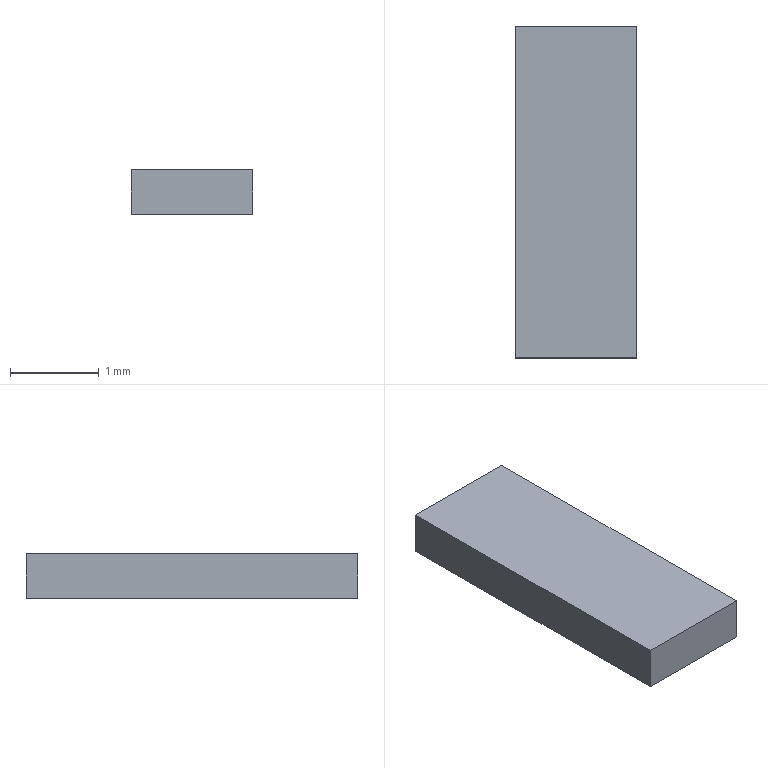Part | SolidWorks | features BaseBody 1 | 1 solid | 6 faces | box 1.375 x 3.75 x 0.5 mm | volume 2.578 mm3 | plane 6
STEP:
#1=CARTESIAN_POINT('',(-6.625,18.625,1.));
#2=VERTEX_POINT('',#1);
#3=CARTESIAN_POINT('',(-6.625,14.875,1.));
#4=VERTEX_POINT('',#3);
#5=CARTESIAN_POINT('',(-6.625,18.625,1.));
#6=DIRECTION('',(0.,-1.,0.));
#7=VECTOR('',#6,1000.);
#8=LINE('',#5,#7);
#9=EDGE_CURVE('',#2,#4,#8,.T.);
#10=ORIENTED_EDGE('',*,*,#9,.T.);
#11=CARTESIAN_POINT('',(-6.625,14.875,1.5));
#12=VERTEX_POINT('',#11);
#13=CARTESIAN_POINT('',(-6.625,14.875,1.5));
#14=DIRECTION('',(0.,0.,-1.));
#15=VECTOR('',#14,1000.);
#16=LINE('',#13,#15);
#17=EDGE_CURVE('',#12,#4,#16,.T.);
#18=ORIENTED_EDGE('',*,*,#17,.F.);
#19=CARTESIAN_POINT('',(-6.625,18.625,1.5));
#20=VERTEX_POINT('',#19);
#21=CARTESIAN_POINT('',(-6.625,18.625,1.5));
#22=DIRECTION('',(0.,-1.,0.));
#23=VECTOR('',#22,1000.);
#24=LINE('',#21,#23);
#25=EDGE_CURVE('',#20,#12,#24,.T.);
#26=ORIENTED_EDGE('',*,*,#25,.F.);
#27=CARTESIAN_POINT('',(-6.625,18.625,1.5));
#28=DIRECTION('',(0.,0.,-1.));
#29=VECTOR('',#28,1000.);
#30=LINE('',#27,#29);
#31=EDGE_CURVE('',#20,#2,#30,.T.);
#32=ORIENTED_EDGE('',*,*,#31,.T.);
#33=EDGE_LOOP('',(#10,#18,#26,#32));
#34=FACE_OUTER_BOUND('',#33,.T.);
#35=CARTESIAN_POINT('',(-6.625,18.625,1.5));
#36=DIRECTION('',(1.,0.,0.));
#37=DIRECTION('',(0.,0.,-1.));
#38=AXIS2_PLACEMENT_3D('',#35,#36,#37);
#39=PLANE('',#38);
#40=ADVANCED_FACE('',(#34),#39,.F.);
#41=CARTESIAN_POINT('',(-5.25,14.875,1.));
#42=VERTEX_POINT('',#41);
#43=CARTESIAN_POINT('',(-6.625,14.875,1.));
#44=DIRECTION('',(1.,0.,0.));
#45=VECTOR('',#44,1000.);
#46=LINE('',#43,#45);
#47=EDGE_CURVE('',#4,#42,#46,.T.);
#48=ORIENTED_EDGE('',*,*,#47,.T.);
#49=CARTESIAN_POINT('',(-5.25,14.875,1.5));
#50=VERTEX_POINT('',#49);
#51=CARTESIAN_POINT('',(-5.25,14.875,1.5));
#52=DIRECTION('',(0.,0.,-1.));
#53=VECTOR('',#52,1000.);
#54=LINE('',#51,#53);
#55=EDGE_CURVE('',#50,#42,#54,.T.);
#56=ORIENTED_EDGE('',*,*,#55,.F.);
#57=CARTESIAN_POINT('',(-6.625,14.875,1.5));
#58=DIRECTION('',(1.,0.,0.));
#59=VECTOR('',#58,1000.);
#60=LINE('',#57,#59);
#61=EDGE_CURVE('',#12,#50,#60,.T.);
#62=ORIENTED_EDGE('',*,*,#61,.F.);
#63=ORIENTED_EDGE('',*,*,#17,.T.);
#64=EDGE_LOOP('',(#48,#56,#62,#63));
#65=FACE_OUTER_BOUND('',#64,.T.);
#66=CARTESIAN_POINT('',(-6.625,14.875,1.5));
#67=DIRECTION('',(0.,1.,0.));
#68=DIRECTION('',(0.,0.,1.));
#69=AXIS2_PLACEMENT_3D('',#66,#67,#68);
#70=PLANE('',#69);
#71=ADVANCED_FACE('',(#65),#70,.F.);
#72=CARTESIAN_POINT('',(-5.25,18.625,1.));
#73=VERTEX_POINT('',#72);
#74=CARTESIAN_POINT('',(-5.25,14.875,1.));
#75=DIRECTION('',(0.,1.,0.));
#76=VECTOR('',#75,1000.);
#77=LINE('',#74,#76);
#78=EDGE_CURVE('',#42,#73,#77,.T.);
#79=ORIENTED_EDGE('',*,*,#78,.T.);
#80=CARTESIAN_POINT('',(-5.25,18.625,1.5));
#81=VERTEX_POINT('',#80);
#82=CARTESIAN_POINT('',(-5.25,18.625,1.5));
#83=DIRECTION('',(0.,0.,-1.));
#84=VECTOR('',#83,1000.);
#85=LINE('',#82,#84);
#86=EDGE_CURVE('',#81,#73,#85,.T.);
#87=ORIENTED_EDGE('',*,*,#86,.F.);
#88=CARTESIAN_POINT('',(-5.25,14.875,1.5));
#89=DIRECTION('',(0.,1.,0.));
#90=VECTOR('',#89,1000.);
#91=LINE('',#88,#90);
#92=EDGE_CURVE('',#50,#81,#91,.T.);
#93=ORIENTED_EDGE('',*,*,#92,.F.);
#94=ORIENTED_EDGE('',*,*,#55,.T.);
#95=EDGE_LOOP('',(#79,#87,#93,#94));
#96=FACE_OUTER_BOUND('',#95,.T.);
#97=CARTESIAN_POINT('',(-5.25,14.875,1.5));
#98=DIRECTION('',(-1.,0.,0.));
#99=DIRECTION('',(0.,-1.,0.));
#100=AXIS2_PLACEMENT_3D('',#97,#98,#99);
#101=PLANE('',#100);
#102=ADVANCED_FACE('',(#96),#101,.F.);
#103=CARTESIAN_POINT('',(-5.25,18.625,1.));
#104=DIRECTION('',(-1.,0.,0.));
#105=VECTOR('',#104,1000.);
#106=LINE('',#103,#105);
#107=EDGE_CURVE('',#73,#2,#106,.T.);
#108=ORIENTED_EDGE('',*,*,#107,.T.);
#109=ORIENTED_EDGE('',*,*,#31,.F.);
#110=CARTESIAN_POINT('',(-5.25,18.625,1.5));
#111=DIRECTION('',(-1.,0.,0.));
#112=VECTOR('',#111,1000.);
#113=LINE('',#110,#112);
#114=EDGE_CURVE('',#81,#20,#113,.T.);
#115=ORIENTED_EDGE('',*,*,#114,.F.);
#116=ORIENTED_EDGE('',*,*,#86,.T.);
#117=EDGE_LOOP('',(#108,#109,#115,#116));
#118=FACE_OUTER_BOUND('',#117,.T.);
#119=CARTESIAN_POINT('',(-5.25,18.625,1.5));
#120=DIRECTION('',(0.,-1.,0.));
#121=DIRECTION('',(0.,0.,-1.));
#122=AXIS2_PLACEMENT_3D('',#119,#120,#121);
#123=PLANE('',#122);
#124=ADVANCED_FACE('',(#118),#123,.F.);
#125=ORIENTED_EDGE('',*,*,#25,.T.);
#126=ORIENTED_EDGE('',*,*,#61,.T.);
#127=ORIENTED_EDGE('',*,*,#92,.T.);
#128=ORIENTED_EDGE('',*,*,#114,.T.);
#129=EDGE_LOOP('',(#125,#126,#127,#128));
#130=FACE_OUTER_BOUND('',#129,.T.);
#131=CARTESIAN_POINT('',(0.,0.,1.5));
#132=DIRECTION('',(0.,0.,1.));
#133=DIRECTION('',(1.,0.,0.));
#134=AXIS2_PLACEMENT_3D('',#131,#132,#133);
#135=PLANE('',#134);
#136=ADVANCED_FACE('',(#130),#135,.T.);
#137=ORIENTED_EDGE('',*,*,#9,.F.);
#138=ORIENTED_EDGE('',*,*,#107,.F.);
#139=ORIENTED_EDGE('',*,*,#78,.F.);
#140=ORIENTED_EDGE('',*,*,#47,.F.);
#141=EDGE_LOOP('',(#137,#138,#139,#140));
#142=FACE_OUTER_BOUND('',#141,.T.);
#143=CARTESIAN_POINT('',(0.,0.,1.));
#144=DIRECTION('',(0.,0.,1.));
#145=DIRECTION('',(1.,0.,0.));
#146=AXIS2_PLACEMENT_3D('',#143,#144,#145);
#147=PLANE('',#146);
#148=ADVANCED_FACE('',(#142),#147,.F.);
#149=CLOSED_SHELL('',(#40,#71,#102,#124,#136,#148));
#150=MANIFOLD_SOLID_BREP('',#149);
#151=CARTESIAN_POINT('',(0.,0.,0.));
#152=DIRECTION('',(0.,0.,1.));
#153=DIRECTION('',(1.,0.,0.));
#154=AXIS2_PLACEMENT_3D('',#151,#152,#153);
#155=(LENGTH_UNIT()NAMED_UNIT(*)SI_UNIT(.MILLI.,.METRE.));
#156=UNCERTAINTY_MEASURE_WITH_UNIT(LENGTH_MEASURE(0.00001),#155,'','');
#157=(NAMED_UNIT(*)PLANE_ANGLE_UNIT()SI_UNIT($,.RADIAN.));
#158=(NAMED_UNIT(*)SI_UNIT($,.STERADIAN.)SOLID_ANGLE_UNIT());
#159=(GEOMETRIC_REPRESENTATION_CONTEXT(3)GLOBAL_UNCERTAINTY_ASSIGNED_CONTEXT((#156))GLOBAL_UNIT_ASSIGNED_CONTEXT((#155,#157,#158))REPRESENTATION_CONTEXT('',''));
#160=ADVANCED_BREP_SHAPE_REPRESENTATION('',(#150,#154),#159);